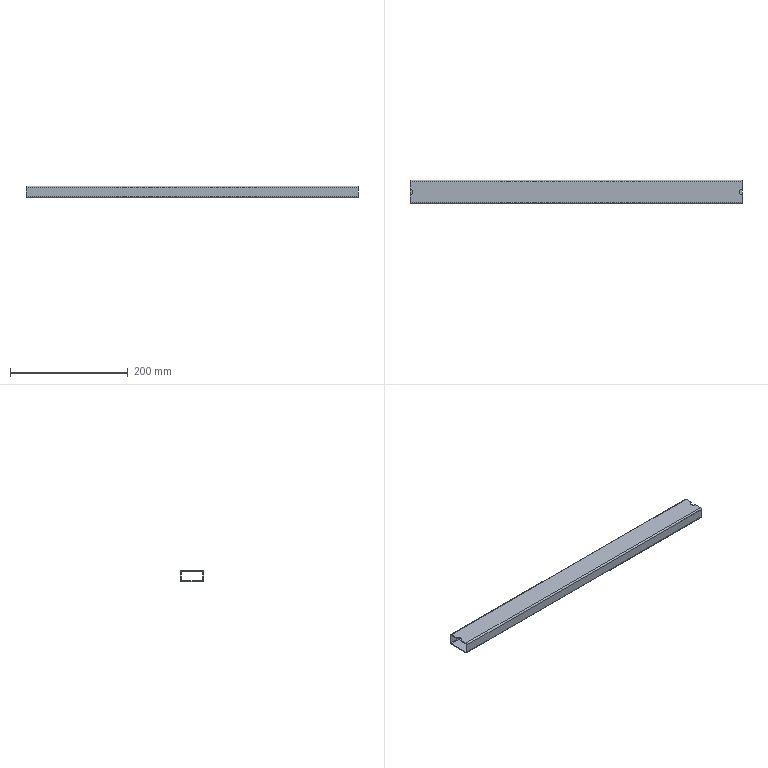Part | STEP file | 7100505 | 1 solid | 20 faces | box 565 x 40 x 20 mm | volume 93951 mm3 | plane 10 | cylinder 10 | commonest cylinder face diameters 2 x4 5 x4 10 x2